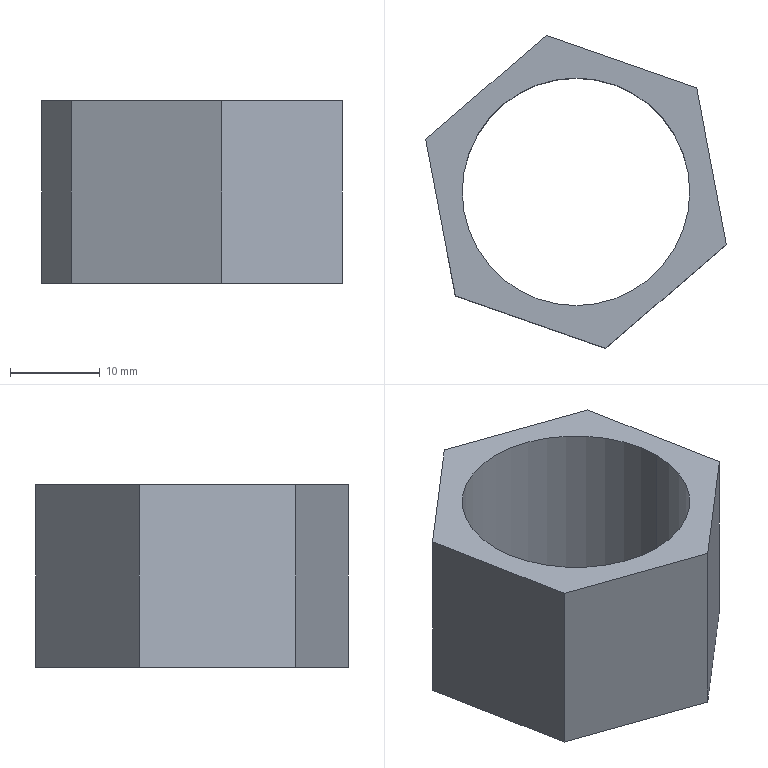Part | SolidWorks | features Extrusion 1, Scale 1 | 1 solid | 10 faces | box 33.572 x 34.936 x 20.32 mm | volume 6393 mm3 | plane 8 | cylinder 2 | commonest cylinder face diameters 25.4 x2
STEP:
#1=CARTESIAN_POINT('',(-12.7,0.,20.32));
#2=VERTEX_POINT('',#1);
#3=CARTESIAN_POINT('',(12.7,0.,20.32));
#4=VERTEX_POINT('',#3);
#5=CARTESIAN_POINT('',(0.,0.,20.32));
#6=DIRECTION('',(0.,0.,1.));
#7=DIRECTION('',(1.,0.,0.));
#8=AXIS2_PLACEMENT_3D('',#5,#6,#7);
#9=CIRCLE('',#8,12.7);
#10=EDGE_CURVE('',#2,#4,#9,.T.);
#11=ORIENTED_EDGE('',*,*,#10,.T.);
#12=CARTESIAN_POINT('',(12.7,0.,0.));
#13=VERTEX_POINT('',#12);
#14=CARTESIAN_POINT('',(12.7,0.,20.32));
#15=DIRECTION('',(0.,0.,-1.));
#16=VECTOR('',#15,1000.);
#17=LINE('',#14,#16);
#18=EDGE_CURVE('',#4,#13,#17,.T.);
#19=ORIENTED_EDGE('',*,*,#18,.T.);
#20=CARTESIAN_POINT('',(-12.7,0.,0.));
#21=VERTEX_POINT('',#20);
#22=CARTESIAN_POINT('',(0.,0.,0.));
#23=DIRECTION('',(0.,0.,1.));
#24=DIRECTION('',(1.,0.,0.));
#25=AXIS2_PLACEMENT_3D('',#22,#23,#24);
#26=CIRCLE('',#25,12.7);
#27=EDGE_CURVE('',#21,#13,#26,.T.);
#28=ORIENTED_EDGE('',*,*,#27,.F.);
#29=CARTESIAN_POINT('',(-12.7,0.,20.32));
#30=DIRECTION('',(0.,0.,-1.));
#31=VECTOR('',#30,1000.);
#32=LINE('',#29,#31);
#33=EDGE_CURVE('',#2,#21,#32,.T.);
#34=ORIENTED_EDGE('',*,*,#33,.F.);
#35=EDGE_LOOP('',(#11,#19,#28,#34));
#36=FACE_OUTER_BOUND('',#35,.T.);
#37=CARTESIAN_POINT('',(0.,0.,20.32));
#38=DIRECTION('',(0.,0.,-1.));
#39=DIRECTION('',(-1.,0.,0.));
#40=AXIS2_PLACEMENT_3D('',#37,#38,#39);
#41=CYLINDRICAL_SURFACE('',#40,12.7);
#42=ADVANCED_FACE('',(#36),#41,.F.);
#43=CARTESIAN_POINT('',(16.786,-5.861,20.32));
#44=VERTEX_POINT('',#43);
#45=CARTESIAN_POINT('',(13.469,11.606,20.32));
#46=VERTEX_POINT('',#45);
#47=CARTESIAN_POINT('',(16.786,-5.861,20.32));
#48=DIRECTION('',(-0.1866,0.9824,0.));
#49=VECTOR('',#48,1000.);
#50=LINE('',#47,#49);
#51=EDGE_CURVE('',#44,#46,#50,.T.);
#52=ORIENTED_EDGE('',*,*,#51,.T.);
#53=CARTESIAN_POINT('',(-3.317,17.468,20.32));
#54=VERTEX_POINT('',#53);
#55=CARTESIAN_POINT('',(13.469,11.606,20.32));
#56=DIRECTION('',(-0.9441,0.3297,0.));
#57=VECTOR('',#56,1000.);
#58=LINE('',#55,#57);
#59=EDGE_CURVE('',#46,#54,#58,.T.);
#60=ORIENTED_EDGE('',*,*,#59,.T.);
#61=CARTESIAN_POINT('',(-16.786,5.861,20.32));
#62=VERTEX_POINT('',#61);
#63=CARTESIAN_POINT('',(-3.317,17.468,20.32));
#64=DIRECTION('',(-0.7575,-0.6528,0.));
#65=VECTOR('',#64,1000.);
#66=LINE('',#63,#65);
#67=EDGE_CURVE('',#54,#62,#66,.T.);
#68=ORIENTED_EDGE('',*,*,#67,.T.);
#69=CARTESIAN_POINT('',(-13.469,-11.606,20.32));
#70=VERTEX_POINT('',#69);
#71=CARTESIAN_POINT('',(-16.786,5.861,20.32));
#72=DIRECTION('',(0.1866,-0.9824,0.));
#73=VECTOR('',#72,1000.);
#74=LINE('',#71,#73);
#75=EDGE_CURVE('',#62,#70,#74,.T.);
#76=ORIENTED_EDGE('',*,*,#75,.T.);
#77=CARTESIAN_POINT('',(3.317,-17.468,20.32));
#78=VERTEX_POINT('',#77);
#79=CARTESIAN_POINT('',(-13.469,-11.606,20.32));
#80=DIRECTION('',(0.9441,-0.3297,0.));
#81=VECTOR('',#80,1000.);
#82=LINE('',#79,#81);
#83=EDGE_CURVE('',#70,#78,#82,.T.);
#84=ORIENTED_EDGE('',*,*,#83,.T.);
#85=CARTESIAN_POINT('',(3.317,-17.468,20.32));
#86=DIRECTION('',(0.7575,0.6528,0.));
#87=VECTOR('',#86,1000.);
#88=LINE('',#85,#87);
#89=EDGE_CURVE('',#78,#44,#88,.T.);
#90=ORIENTED_EDGE('',*,*,#89,.T.);
#91=EDGE_LOOP('',(#52,#60,#68,#76,#84,#90));
#92=FACE_OUTER_BOUND('',#91,.T.);
#93=ORIENTED_EDGE('',*,*,#10,.F.);
#94=CARTESIAN_POINT('',(0.,0.,20.32));
#95=DIRECTION('',(0.,0.,1.));
#96=DIRECTION('',(1.,0.,0.));
#97=AXIS2_PLACEMENT_3D('',#94,#95,#96);
#98=CIRCLE('',#97,12.7);
#99=EDGE_CURVE('',#4,#2,#98,.T.);
#100=ORIENTED_EDGE('',*,*,#99,.F.);
#101=EDGE_LOOP('',(#93,#100));
#102=FACE_BOUND('',#101,.T.);
#103=CARTESIAN_POINT('',(0.,0.,20.32));
#104=DIRECTION('',(0.,0.,1.));
#105=DIRECTION('',(1.,0.,0.));
#106=AXIS2_PLACEMENT_3D('',#103,#104,#105);
#107=PLANE('',#106);
#108=ADVANCED_FACE('',(#92,#102),#107,.T.);
#109=CARTESIAN_POINT('',(16.786,-5.861,0.));
#110=VERTEX_POINT('',#109);
#111=CARTESIAN_POINT('',(13.469,11.606,0.));
#112=VERTEX_POINT('',#111);
#113=CARTESIAN_POINT('',(16.786,-5.861,0.));
#114=DIRECTION('',(-0.1866,0.9824,0.));
#115=VECTOR('',#114,1000.);
#116=LINE('',#113,#115);
#117=EDGE_CURVE('',#110,#112,#116,.T.);
#118=ORIENTED_EDGE('',*,*,#117,.F.);
#119=CARTESIAN_POINT('',(3.317,-17.468,0.));
#120=VERTEX_POINT('',#119);
#121=CARTESIAN_POINT('',(3.317,-17.468,0.));
#122=DIRECTION('',(0.7575,0.6528,0.));
#123=VECTOR('',#122,1000.);
#124=LINE('',#121,#123);
#125=EDGE_CURVE('',#120,#110,#124,.T.);
#126=ORIENTED_EDGE('',*,*,#125,.F.);
#127=CARTESIAN_POINT('',(-13.469,-11.606,0.));
#128=VERTEX_POINT('',#127);
#129=CARTESIAN_POINT('',(-13.469,-11.606,0.));
#130=DIRECTION('',(0.9441,-0.3297,0.));
#131=VECTOR('',#130,1000.);
#132=LINE('',#129,#131);
#133=EDGE_CURVE('',#128,#120,#132,.T.);
#134=ORIENTED_EDGE('',*,*,#133,.F.);
#135=CARTESIAN_POINT('',(-16.786,5.861,0.));
#136=VERTEX_POINT('',#135);
#137=CARTESIAN_POINT('',(-16.786,5.861,0.));
#138=DIRECTION('',(0.1866,-0.9824,0.));
#139=VECTOR('',#138,1000.);
#140=LINE('',#137,#139);
#141=EDGE_CURVE('',#136,#128,#140,.T.);
#142=ORIENTED_EDGE('',*,*,#141,.F.);
#143=CARTESIAN_POINT('',(-3.317,17.468,0.));
#144=VERTEX_POINT('',#143);
#145=CARTESIAN_POINT('',(-3.317,17.468,0.));
#146=DIRECTION('',(-0.7575,-0.6528,0.));
#147=VECTOR('',#146,1000.);
#148=LINE('',#145,#147);
#149=EDGE_CURVE('',#144,#136,#148,.T.);
#150=ORIENTED_EDGE('',*,*,#149,.F.);
#151=CARTESIAN_POINT('',(13.469,11.606,0.));
#152=DIRECTION('',(-0.9441,0.3297,0.));
#153=VECTOR('',#152,1000.);
#154=LINE('',#151,#153);
#155=EDGE_CURVE('',#112,#144,#154,.T.);
#156=ORIENTED_EDGE('',*,*,#155,.F.);
#157=EDGE_LOOP('',(#118,#126,#134,#142,#150,#156));
#158=FACE_OUTER_BOUND('',#157,.T.);
#159=ORIENTED_EDGE('',*,*,#27,.T.);
#160=CARTESIAN_POINT('',(0.,0.,0.));
#161=DIRECTION('',(0.,0.,1.));
#162=DIRECTION('',(1.,0.,0.));
#163=AXIS2_PLACEMENT_3D('',#160,#161,#162);
#164=CIRCLE('',#163,12.7);
#165=EDGE_CURVE('',#13,#21,#164,.T.);
#166=ORIENTED_EDGE('',*,*,#165,.T.);
#167=EDGE_LOOP('',(#159,#166));
#168=FACE_BOUND('',#167,.T.);
#169=CARTESIAN_POINT('',(0.,0.,0.));
#170=DIRECTION('',(0.,0.,1.));
#171=DIRECTION('',(1.,0.,0.));
#172=AXIS2_PLACEMENT_3D('',#169,#170,#171);
#173=PLANE('',#172);
#174=ADVANCED_FACE('',(#158,#168),#173,.F.);
#175=ORIENTED_EDGE('',*,*,#117,.T.);
#176=CARTESIAN_POINT('',(13.469,11.606,20.32));
#177=DIRECTION('',(0.,0.,-1.));
#178=VECTOR('',#177,1000.);
#179=LINE('',#176,#178);
#180=EDGE_CURVE('',#46,#112,#179,.T.);
#181=ORIENTED_EDGE('',*,*,#180,.F.);
#182=ORIENTED_EDGE('',*,*,#51,.F.);
#183=CARTESIAN_POINT('',(16.786,-5.861,20.32));
#184=DIRECTION('',(0.,0.,-1.));
#185=VECTOR('',#184,1000.);
#186=LINE('',#183,#185);
#187=EDGE_CURVE('',#44,#110,#186,.T.);
#188=ORIENTED_EDGE('',*,*,#187,.T.);
#189=EDGE_LOOP('',(#175,#181,#182,#188));
#190=FACE_OUTER_BOUND('',#189,.T.);
#191=CARTESIAN_POINT('',(16.786,-5.861,20.32));
#192=DIRECTION('',(-0.9824,-0.1866,0.));
#193=DIRECTION('',(0.1866,-0.9824,0.));
#194=AXIS2_PLACEMENT_3D('',#191,#192,#193);
#195=PLANE('',#194);
#196=ADVANCED_FACE('',(#190),#195,.F.);
#197=ORIENTED_EDGE('',*,*,#155,.T.);
#198=CARTESIAN_POINT('',(-3.317,17.468,20.32));
#199=DIRECTION('',(0.,0.,-1.));
#200=VECTOR('',#199,1000.);
#201=LINE('',#198,#200);
#202=EDGE_CURVE('',#54,#144,#201,.T.);
#203=ORIENTED_EDGE('',*,*,#202,.F.);
#204=ORIENTED_EDGE('',*,*,#59,.F.);
#205=ORIENTED_EDGE('',*,*,#180,.T.);
#206=EDGE_LOOP('',(#197,#203,#204,#205));
#207=FACE_OUTER_BOUND('',#206,.T.);
#208=CARTESIAN_POINT('',(13.469,11.606,20.32));
#209=DIRECTION('',(-0.3297,-0.9441,0.));
#210=DIRECTION('',(0.9441,-0.3297,0.));
#211=AXIS2_PLACEMENT_3D('',#208,#209,#210);
#212=PLANE('',#211);
#213=ADVANCED_FACE('',(#207),#212,.F.);
#214=ORIENTED_EDGE('',*,*,#149,.T.);
#215=CARTESIAN_POINT('',(-16.786,5.861,20.32));
#216=DIRECTION('',(0.,0.,-1.));
#217=VECTOR('',#216,1000.);
#218=LINE('',#215,#217);
#219=EDGE_CURVE('',#62,#136,#218,.T.);
#220=ORIENTED_EDGE('',*,*,#219,.F.);
#221=ORIENTED_EDGE('',*,*,#67,.F.);
#222=ORIENTED_EDGE('',*,*,#202,.T.);
#223=EDGE_LOOP('',(#214,#220,#221,#222));
#224=FACE_OUTER_BOUND('',#223,.T.);
#225=CARTESIAN_POINT('',(-3.317,17.468,20.32));
#226=DIRECTION('',(0.6528,-0.7575,0.));
#227=DIRECTION('',(0.7575,0.6528,0.));
#228=AXIS2_PLACEMENT_3D('',#225,#226,#227);
#229=PLANE('',#228);
#230=ADVANCED_FACE('',(#224),#229,.F.);
#231=ORIENTED_EDGE('',*,*,#141,.T.);
#232=CARTESIAN_POINT('',(-13.469,-11.606,20.32));
#233=DIRECTION('',(0.,0.,-1.));
#234=VECTOR('',#233,1000.);
#235=LINE('',#232,#234);
#236=EDGE_CURVE('',#70,#128,#235,.T.);
#237=ORIENTED_EDGE('',*,*,#236,.F.);
#238=ORIENTED_EDGE('',*,*,#75,.F.);
#239=ORIENTED_EDGE('',*,*,#219,.T.);
#240=EDGE_LOOP('',(#231,#237,#238,#239));
#241=FACE_OUTER_BOUND('',#240,.T.);
#242=CARTESIAN_POINT('',(-16.786,5.861,20.32));
#243=DIRECTION('',(0.9824,0.1866,0.));
#244=DIRECTION('',(-0.1866,0.9824,0.));
#245=AXIS2_PLACEMENT_3D('',#242,#243,#244);
#246=PLANE('',#245);
#247=ADVANCED_FACE('',(#241),#246,.F.);
#248=ORIENTED_EDGE('',*,*,#133,.T.);
#249=CARTESIAN_POINT('',(3.317,-17.468,20.32));
#250=DIRECTION('',(0.,0.,-1.));
#251=VECTOR('',#250,1000.);
#252=LINE('',#249,#251);
#253=EDGE_CURVE('',#78,#120,#252,.T.);
#254=ORIENTED_EDGE('',*,*,#253,.F.);
#255=ORIENTED_EDGE('',*,*,#83,.F.);
#256=ORIENTED_EDGE('',*,*,#236,.T.);
#257=EDGE_LOOP('',(#248,#254,#255,#256));
#258=FACE_OUTER_BOUND('',#257,.T.);
#259=CARTESIAN_POINT('',(-13.469,-11.606,20.32));
#260=DIRECTION('',(0.3297,0.9441,0.));
#261=DIRECTION('',(-0.9441,0.3297,0.));
#262=AXIS2_PLACEMENT_3D('',#259,#260,#261);
#263=PLANE('',#262);
#264=ADVANCED_FACE('',(#258),#263,.F.);
#265=ORIENTED_EDGE('',*,*,#125,.T.);
#266=ORIENTED_EDGE('',*,*,#187,.F.);
#267=ORIENTED_EDGE('',*,*,#89,.F.);
#268=ORIENTED_EDGE('',*,*,#253,.T.);
#269=EDGE_LOOP('',(#265,#266,#267,#268));
#270=FACE_OUTER_BOUND('',#269,.T.);
#271=CARTESIAN_POINT('',(3.317,-17.468,20.32));
#272=DIRECTION('',(-0.6528,0.7575,0.));
#273=DIRECTION('',(-0.7575,-0.6528,0.));
#274=AXIS2_PLACEMENT_3D('',#271,#272,#273);
#275=PLANE('',#274);
#276=ADVANCED_FACE('',(#270),#275,.F.);
#277=ORIENTED_EDGE('',*,*,#18,.F.);
#278=ORIENTED_EDGE('',*,*,#99,.T.);
#279=ORIENTED_EDGE('',*,*,#33,.T.);
#280=ORIENTED_EDGE('',*,*,#165,.F.);
#281=EDGE_LOOP('',(#277,#278,#279,#280));
#282=FACE_OUTER_BOUND('',#281,.T.);
#283=CARTESIAN_POINT('',(0.,0.,20.32));
#284=DIRECTION('',(0.,0.,-1.));
#285=DIRECTION('',(-1.,0.,0.));
#286=AXIS2_PLACEMENT_3D('',#283,#284,#285);
#287=CYLINDRICAL_SURFACE('',#286,12.7);
#288=ADVANCED_FACE('',(#282),#287,.F.);
#289=CLOSED_SHELL('',(#42,#108,#174,#196,#213,#230,#247,#264,#276,#288));
#290=MANIFOLD_SOLID_BREP('',#289);
#291=CARTESIAN_POINT('',(0.,0.,0.));
#292=DIRECTION('',(0.,0.,1.));
#293=DIRECTION('',(1.,0.,0.));
#294=AXIS2_PLACEMENT_3D('',#291,#292,#293);
#295=(LENGTH_UNIT()NAMED_UNIT(*)SI_UNIT(.MILLI.,.METRE.));
#296=UNCERTAINTY_MEASURE_WITH_UNIT(LENGTH_MEASURE(0.00001),#295,'','');
#297=(NAMED_UNIT(*)PLANE_ANGLE_UNIT()SI_UNIT($,.RADIAN.));
#298=(NAMED_UNIT(*)SI_UNIT($,.STERADIAN.)SOLID_ANGLE_UNIT());
#299=(GEOMETRIC_REPRESENTATION_CONTEXT(3)GLOBAL_UNCERTAINTY_ASSIGNED_CONTEXT((#296))GLOBAL_UNIT_ASSIGNED_CONTEXT((#295,#297,#298))REPRESENTATION_CONTEXT('',''));
#300=ADVANCED_BREP_SHAPE_REPRESENTATION('',(#290,#294),#299);